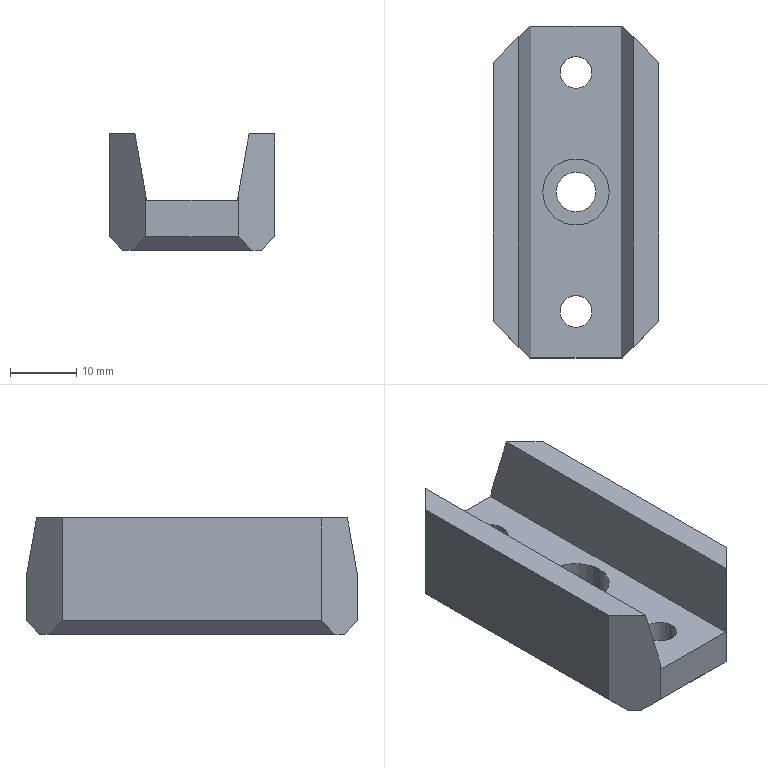Part | Creo | 1 solid | 27 faces | box 25 x 50 x 17.5 mm | volume 12117 mm3 | plane 19 | cylinder 8 | commonest cylinder face diameters 4.8 x4 6 x2 10 x2
STEP:
#1=CARTESIAN_POINT('',(-137.,25.,29.153));
#2=VERTEX_POINT('',#1);
#3=CARTESIAN_POINT('',(-136.825,25.,28.161));
#4=VERTEX_POINT('',#3);
#5=CARTESIAN_POINT('',(-137.,25.,29.153));
#6=DIRECTION('',(0.1736,0.,-0.9848));
#7=VECTOR('',#6,1.008);
#8=LINE('',#5,#7);
#9=EDGE_CURVE('',#2,#4,#8,.T.);
#10=ORIENTED_EDGE('',*,*,#9,.T.);
#11=CARTESIAN_POINT('',(-136.825,-25.,28.161));
#12=VERTEX_POINT('',#11);
#13=CARTESIAN_POINT('',(-136.825,-25.,28.161));
#14=DIRECTION('',(0.,1.,0.));
#15=VECTOR('',#14,50.);
#16=LINE('',#13,#15);
#17=EDGE_CURVE('',#12,#4,#16,.T.);
#18=ORIENTED_EDGE('',*,*,#17,.F.);
#19=CARTESIAN_POINT('',(-137.,-25.,29.153));
#20=VERTEX_POINT('',#19);
#21=CARTESIAN_POINT('',(-136.825,-25.,28.161));
#22=DIRECTION('',(-0.1736,0.,0.9848));
#23=VECTOR('',#22,1.008);
#24=LINE('',#21,#23);
#25=EDGE_CURVE('',#12,#20,#24,.T.);
#26=ORIENTED_EDGE('',*,*,#25,.T.);
#27=CARTESIAN_POINT('',(-138.588,-23.412,38.161));
#28=VERTEX_POINT('',#27);
#29=CARTESIAN_POINT('',(-138.588,-23.412,38.161));
#30=DIRECTION('',(0.1711,-0.1711,-0.9703));
#31=VECTOR('',#30,9.283);
#32=LINE('',#29,#31);
#33=EDGE_CURVE('',#28,#20,#32,.T.);
#34=ORIENTED_EDGE('',*,*,#33,.F.);
#35=CARTESIAN_POINT('',(-138.588,23.412,38.161));
#36=VERTEX_POINT('',#35);
#37=CARTESIAN_POINT('',(-138.588,-23.412,38.161));
#38=DIRECTION('',(0.,1.,0.));
#39=VECTOR('',#38,46.823);
#40=LINE('',#37,#39);
#41=EDGE_CURVE('',#28,#36,#40,.T.);
#42=ORIENTED_EDGE('',*,*,#41,.T.);
#43=CARTESIAN_POINT('',(-137.,25.,29.153));
#44=DIRECTION('',(-0.1711,-0.1711,0.9703));
#45=VECTOR('',#44,9.283);
#46=LINE('',#43,#45);
#47=EDGE_CURVE('',#2,#36,#46,.T.);
#48=ORIENTED_EDGE('',*,*,#47,.F.);
#49=EDGE_LOOP('',(#10,#18,#26,#34,#42,#48));
#50=FACE_OUTER_BOUND('',#49,.F.);
#51=CARTESIAN_POINT('',(-136.825,50.,28.161));
#52=DIRECTION('',(0.9848,0.,0.1736));
#53=DIRECTION('',(-0.1736,0.,0.9848));
#54=AXIS2_PLACEMENT_3D('',#51,#52,#53);
#55=PLANE('',#54);
#56=ADVANCED_FACE('',(#50),#55,.T.);
#57=CARTESIAN_POINT('',(-123.175,25.,28.161));
#58=VERTEX_POINT('',#57);
#59=CARTESIAN_POINT('',(-123.175,25.,28.161));
#60=DIRECTION('',(-1.,0.,0.));
#61=VECTOR('',#60,13.65);
#62=LINE('',#59,#61);
#63=EDGE_CURVE('',#58,#4,#62,.T.);
#64=ORIENTED_EDGE('',*,*,#63,.T.);
#65=ORIENTED_EDGE('',*,*,#9,.F.);
#66=CARTESIAN_POINT('',(-137.,25.,22.661));
#67=VERTEX_POINT('',#66);
#68=CARTESIAN_POINT('',(-137.,25.,29.153));
#69=DIRECTION('',(0.,0.,-1.));
#70=VECTOR('',#69,6.492);
#71=LINE('',#68,#70);
#72=EDGE_CURVE('',#2,#67,#71,.T.);
#73=ORIENTED_EDGE('',*,*,#72,.T.);
#74=CARTESIAN_POINT('',(-123.,25.,22.661));
#75=VERTEX_POINT('',#74);
#76=CARTESIAN_POINT('',(-137.,25.,22.661));
#77=DIRECTION('',(1.,0.,0.));
#78=VECTOR('',#77,14.);
#79=LINE('',#76,#78);
#80=EDGE_CURVE('',#67,#75,#79,.T.);
#81=ORIENTED_EDGE('',*,*,#80,.T.);
#82=CARTESIAN_POINT('',(-123.,25.,29.153));
#83=VERTEX_POINT('',#82);
#84=CARTESIAN_POINT('',(-123.,25.,22.661));
#85=DIRECTION('',(0.,0.,1.));
#86=VECTOR('',#85,6.492);
#87=LINE('',#84,#86);
#88=EDGE_CURVE('',#75,#83,#87,.T.);
#89=ORIENTED_EDGE('',*,*,#88,.T.);
#90=CARTESIAN_POINT('',(-123.175,25.,28.161));
#91=DIRECTION('',(0.1736,0.,0.9848));
#92=VECTOR('',#91,1.008);
#93=LINE('',#90,#92);
#94=EDGE_CURVE('',#58,#83,#93,.T.);
#95=ORIENTED_EDGE('',*,*,#94,.F.);
#96=EDGE_LOOP('',(#64,#65,#73,#81,#89,#95));
#97=FACE_OUTER_BOUND('',#96,.F.);
#98=CARTESIAN_POINT('',(-117.5,25.,46.161));
#99=DIRECTION('',(0.,1.,0.));
#100=DIRECTION('',(-1.,0.,0.));
#101=AXIS2_PLACEMENT_3D('',#98,#99,#100);
#102=PLANE('',#101);
#103=ADVANCED_FACE('',(#97),#102,.T.);
#104=ORIENTED_EDGE('',*,*,#17,.T.);
#105=ORIENTED_EDGE('',*,*,#63,.F.);
#106=CARTESIAN_POINT('',(-123.175,-25.,28.161));
#107=VERTEX_POINT('',#106);
#108=CARTESIAN_POINT('',(-123.175,-25.,28.161));
#109=DIRECTION('',(0.,1.,0.));
#110=VECTOR('',#109,50.);
#111=LINE('',#108,#110);
#112=EDGE_CURVE('',#107,#58,#111,.T.);
#113=ORIENTED_EDGE('',*,*,#112,.F.);
#114=CARTESIAN_POINT('',(-123.175,-25.,28.161));
#115=DIRECTION('',(-1.,0.,0.));
#116=VECTOR('',#115,13.65);
#117=LINE('',#114,#116);
#118=EDGE_CURVE('',#107,#12,#117,.T.);
#119=ORIENTED_EDGE('',*,*,#118,.T.);
#120=EDGE_LOOP('',(#104,#105,#113,#119));
#121=FACE_OUTER_BOUND('',#120,.F.);
#122=CARTESIAN_POINT('',(-132.4,18.,28.161));
#123=VERTEX_POINT('',#122);
#124=CARTESIAN_POINT('',(-127.6,18.,28.161));
#125=VERTEX_POINT('',#124);
#126=CARTESIAN_POINT('',(-130.,18.,28.161));
#127=DIRECTION('',(0.,0.,-1.));
#128=DIRECTION('',(-1.,0.,0.));
#129=AXIS2_PLACEMENT_3D('',#126,#127,#128);
#130=CIRCLE('',#129,2.4);
#131=EDGE_CURVE('',#123,#125,#130,.T.);
#132=ORIENTED_EDGE('',*,*,#131,.F.);
#133=CARTESIAN_POINT('',(-130.,18.,28.161));
#134=DIRECTION('',(0.,0.,-1.));
#135=DIRECTION('',(1.,0.,0.));
#136=AXIS2_PLACEMENT_3D('',#133,#134,#135);
#137=CIRCLE('',#136,2.4);
#138=EDGE_CURVE('',#125,#123,#137,.T.);
#139=ORIENTED_EDGE('',*,*,#138,.F.);
#140=EDGE_LOOP('',(#132,#139));
#141=FACE_BOUND('',#140,.F.);
#142=CARTESIAN_POINT('',(-132.4,-18.,28.161));
#143=VERTEX_POINT('',#142);
#144=CARTESIAN_POINT('',(-127.6,-18.,28.161));
#145=VERTEX_POINT('',#144);
#146=CARTESIAN_POINT('',(-130.,-18.,28.161));
#147=DIRECTION('',(0.,0.,-1.));
#148=DIRECTION('',(-1.,0.,0.));
#149=AXIS2_PLACEMENT_3D('',#146,#147,#148);
#150=CIRCLE('',#149,2.4);
#151=EDGE_CURVE('',#143,#145,#150,.T.);
#152=ORIENTED_EDGE('',*,*,#151,.F.);
#153=CARTESIAN_POINT('',(-130.,-18.,28.161));
#154=DIRECTION('',(0.,0.,-1.));
#155=DIRECTION('',(1.,0.,0.));
#156=AXIS2_PLACEMENT_3D('',#153,#154,#155);
#157=CIRCLE('',#156,2.4);
#158=EDGE_CURVE('',#145,#143,#157,.T.);
#159=ORIENTED_EDGE('',*,*,#158,.F.);
#160=EDGE_LOOP('',(#152,#159));
#161=FACE_BOUND('',#160,.F.);
#162=CARTESIAN_POINT('',(-125.,0.,28.161));
#163=VERTEX_POINT('',#162);
#164=CARTESIAN_POINT('',(-135.,0.,28.161));
#165=VERTEX_POINT('',#164);
#166=CARTESIAN_POINT('',(-130.,0.,28.161));
#167=DIRECTION('',(0.,0.,-1.));
#168=DIRECTION('',(1.,0.,0.));
#169=AXIS2_PLACEMENT_3D('',#166,#167,#168);
#170=CIRCLE('',#169,5.);
#171=EDGE_CURVE('',#163,#165,#170,.T.);
#172=ORIENTED_EDGE('',*,*,#171,.F.);
#173=CARTESIAN_POINT('',(-130.,0.,28.161));
#174=DIRECTION('',(0.,0.,-1.));
#175=DIRECTION('',(-1.,0.,0.));
#176=AXIS2_PLACEMENT_3D('',#173,#174,#175);
#177=CIRCLE('',#176,5.);
#178=EDGE_CURVE('',#165,#163,#177,.T.);
#179=ORIENTED_EDGE('',*,*,#178,.F.);
#180=EDGE_LOOP('',(#172,#179));
#181=FACE_BOUND('',#180,.F.);
#182=CARTESIAN_POINT('',(-123.175,50.,28.161));
#183=DIRECTION('',(0.,0.,1.));
#184=DIRECTION('',(-1.,0.,0.));
#185=AXIS2_PLACEMENT_3D('',#182,#183,#184);
#186=PLANE('',#185);
#187=ADVANCED_FACE('',(#121,#141,#161,#181),#186,.T.);
#188=CARTESIAN_POINT('',(-135.,0.,22.161));
#189=VERTEX_POINT('',#188);
#190=CARTESIAN_POINT('',(-125.,0.,22.161));
#191=VERTEX_POINT('',#190);
#192=CARTESIAN_POINT('',(-130.,0.,22.161));
#193=DIRECTION('',(0.,0.,1.));
#194=DIRECTION('',(-1.,0.,0.));
#195=AXIS2_PLACEMENT_3D('',#192,#193,#194);
#196=CIRCLE('',#195,5.);
#197=EDGE_CURVE('',#189,#191,#196,.T.);
#198=ORIENTED_EDGE('',*,*,#197,.T.);
#199=CARTESIAN_POINT('',(-125.,0.,28.161));
#200=DIRECTION('',(0.,0.,-1.));
#201=VECTOR('',#200,6.);
#202=LINE('',#199,#201);
#203=EDGE_CURVE('',#163,#191,#202,.T.);
#204=ORIENTED_EDGE('',*,*,#203,.F.);
#205=ORIENTED_EDGE('',*,*,#171,.T.);
#206=CARTESIAN_POINT('',(-135.,0.,28.161));
#207=DIRECTION('',(0.,0.,-1.));
#208=VECTOR('',#207,6.);
#209=LINE('',#206,#208);
#210=EDGE_CURVE('',#165,#189,#209,.T.);
#211=ORIENTED_EDGE('',*,*,#210,.T.);
#212=EDGE_LOOP('',(#198,#204,#205,#211));
#213=FACE_OUTER_BOUND('',#212,.F.);
#214=CARTESIAN_POINT('',(-130.,0.,28.161));
#215=DIRECTION('',(0.,0.,-1.));
#216=DIRECTION('',(1.,0.,0.));
#217=AXIS2_PLACEMENT_3D('',#214,#215,#216);
#218=CYLINDRICAL_SURFACE('',#217,5.);
#219=ADVANCED_FACE('',(#213),#218,.F.);
#220=CARTESIAN_POINT('',(-130.,0.,22.161));
#221=DIRECTION('',(0.,0.,1.));
#222=DIRECTION('',(1.,0.,0.));
#223=AXIS2_PLACEMENT_3D('',#220,#221,#222);
#224=CIRCLE('',#223,5.);
#225=EDGE_CURVE('',#191,#189,#224,.T.);
#226=ORIENTED_EDGE('',*,*,#225,.F.);
#227=ORIENTED_EDGE('',*,*,#197,.F.);
#228=EDGE_LOOP('',(#226,#227));
#229=FACE_OUTER_BOUND('',#228,.F.);
#230=CARTESIAN_POINT('',(-127.,0.,22.161));
#231=VERTEX_POINT('',#230);
#232=CARTESIAN_POINT('',(-133.,0.,22.161));
#233=VERTEX_POINT('',#232);
#234=CARTESIAN_POINT('',(-130.,0.,22.161));
#235=DIRECTION('',(0.,0.,-1.));
#236=DIRECTION('',(1.,0.,0.));
#237=AXIS2_PLACEMENT_3D('',#234,#235,#236);
#238=CIRCLE('',#237,3.);
#239=EDGE_CURVE('',#231,#233,#238,.T.);
#240=ORIENTED_EDGE('',*,*,#239,.F.);
#241=CARTESIAN_POINT('',(-130.,0.,22.161));
#242=DIRECTION('',(0.,0.,-1.));
#243=DIRECTION('',(-1.,0.,0.));
#244=AXIS2_PLACEMENT_3D('',#241,#242,#243);
#245=CIRCLE('',#244,3.);
#246=EDGE_CURVE('',#233,#231,#245,.T.);
#247=ORIENTED_EDGE('',*,*,#246,.F.);
#248=EDGE_LOOP('',(#240,#247));
#249=FACE_BOUND('',#248,.F.);
#250=CARTESIAN_POINT('',(-130.,0.,22.161));
#251=DIRECTION('',(0.,0.,-1.));
#252=DIRECTION('',(1.,0.,0.));
#253=AXIS2_PLACEMENT_3D('',#250,#251,#252);
#254=PLANE('',#253);
#255=ADVANCED_FACE('',(#229,#249),#254,.F.);
#256=ORIENTED_EDGE('',*,*,#225,.T.);
#257=ORIENTED_EDGE('',*,*,#210,.F.);
#258=ORIENTED_EDGE('',*,*,#178,.T.);
#259=ORIENTED_EDGE('',*,*,#203,.T.);
#260=EDGE_LOOP('',(#256,#257,#258,#259));
#261=FACE_OUTER_BOUND('',#260,.F.);
#262=CARTESIAN_POINT('',(-130.,0.,28.161));
#263=DIRECTION('',(0.,0.,-1.));
#264=DIRECTION('',(1.,0.,0.));
#265=AXIS2_PLACEMENT_3D('',#262,#263,#264);
#266=CYLINDRICAL_SURFACE('',#265,5.);
#267=ADVANCED_FACE('',(#261),#266,.F.);
#268=ORIENTED_EDGE('',*,*,#239,.T.);
#269=CARTESIAN_POINT('',(-133.,0.,20.661));
#270=VERTEX_POINT('',#269);
#271=CARTESIAN_POINT('',(-133.,0.,22.161));
#272=DIRECTION('',(0.,0.,-1.));
#273=VECTOR('',#272,1.5);
#274=LINE('',#271,#273);
#275=EDGE_CURVE('',#233,#270,#274,.T.);
#276=ORIENTED_EDGE('',*,*,#275,.T.);
#277=CARTESIAN_POINT('',(-127.,0.,20.661));
#278=VERTEX_POINT('',#277);
#279=CARTESIAN_POINT('',(-130.,0.,20.661));
#280=DIRECTION('',(0.,0.,1.));
#281=DIRECTION('',(-1.,0.,0.));
#282=AXIS2_PLACEMENT_3D('',#279,#280,#281);
#283=CIRCLE('',#282,3.);
#284=EDGE_CURVE('',#270,#278,#283,.T.);
#285=ORIENTED_EDGE('',*,*,#284,.T.);
#286=CARTESIAN_POINT('',(-127.,0.,22.161));
#287=DIRECTION('',(0.,0.,-1.));
#288=VECTOR('',#287,1.5);
#289=LINE('',#286,#288);
#290=EDGE_CURVE('',#231,#278,#289,.T.);
#291=ORIENTED_EDGE('',*,*,#290,.F.);
#292=EDGE_LOOP('',(#268,#276,#285,#291));
#293=FACE_OUTER_BOUND('',#292,.F.);
#294=CARTESIAN_POINT('',(-130.,0.,46.161));
#295=DIRECTION('',(0.,0.,-1.));
#296=DIRECTION('',(1.,0.,0.));
#297=AXIS2_PLACEMENT_3D('',#294,#295,#296);
#298=CYLINDRICAL_SURFACE('',#297,3.);
#299=ADVANCED_FACE('',(#293),#298,.F.);
#300=ORIENTED_EDGE('',*,*,#246,.T.);
#301=ORIENTED_EDGE('',*,*,#290,.T.);
#302=CARTESIAN_POINT('',(-130.,0.,20.661));
#303=DIRECTION('',(0.,0.,1.));
#304=DIRECTION('',(1.,0.,0.));
#305=AXIS2_PLACEMENT_3D('',#302,#303,#304);
#306=CIRCLE('',#305,3.);
#307=EDGE_CURVE('',#278,#270,#306,.T.);
#308=ORIENTED_EDGE('',*,*,#307,.T.);
#309=ORIENTED_EDGE('',*,*,#275,.F.);
#310=EDGE_LOOP('',(#300,#301,#308,#309));
#311=FACE_OUTER_BOUND('',#310,.F.);
#312=CARTESIAN_POINT('',(-130.,0.,46.161));
#313=DIRECTION('',(0.,0.,-1.));
#314=DIRECTION('',(1.,0.,0.));
#315=AXIS2_PLACEMENT_3D('',#312,#313,#314);
#316=CYLINDRICAL_SURFACE('',#315,3.);
#317=ADVANCED_FACE('',(#311),#316,.F.);
#318=CARTESIAN_POINT('',(-121.,23.,20.661));
#319=VERTEX_POINT('',#318);
#320=CARTESIAN_POINT('',(-139.,23.,20.661));
#321=VERTEX_POINT('',#320);
#322=CARTESIAN_POINT('',(-121.,23.,20.661));
#323=DIRECTION('',(-1.,0.,0.));
#324=VECTOR('',#323,18.);
#325=LINE('',#322,#324);
#326=EDGE_CURVE('',#319,#321,#325,.T.);
#327=ORIENTED_EDGE('',*,*,#326,.T.);
#328=CARTESIAN_POINT('',(-140.5,21.5,20.661));
#329=VERTEX_POINT('',#328);
#330=CARTESIAN_POINT('',(-140.5,21.5,20.661));
#331=DIRECTION('',(0.7071,0.7071,0.));
#332=VECTOR('',#331,2.121);
#333=LINE('',#330,#332);
#334=EDGE_CURVE('',#329,#321,#333,.T.);
#335=ORIENTED_EDGE('',*,*,#334,.F.);
#336=CARTESIAN_POINT('',(-140.5,-21.5,20.661));
#337=VERTEX_POINT('',#336);
#338=CARTESIAN_POINT('',(-140.5,21.5,20.661));
#339=DIRECTION('',(0.,-1.,0.));
#340=VECTOR('',#339,43.);
#341=LINE('',#338,#340);
#342=EDGE_CURVE('',#329,#337,#341,.T.);
#343=ORIENTED_EDGE('',*,*,#342,.T.);
#344=CARTESIAN_POINT('',(-139.,-23.,20.661));
#345=VERTEX_POINT('',#344);
#346=CARTESIAN_POINT('',(-139.,-23.,20.661));
#347=DIRECTION('',(-0.7071,0.7071,0.));
#348=VECTOR('',#347,2.121);
#349=LINE('',#346,#348);
#350=EDGE_CURVE('',#345,#337,#349,.T.);
#351=ORIENTED_EDGE('',*,*,#350,.F.);
#352=CARTESIAN_POINT('',(-121.,-23.,20.661));
#353=VERTEX_POINT('',#352);
#354=CARTESIAN_POINT('',(-139.,-23.,20.661));
#355=DIRECTION('',(1.,0.,0.));
#356=VECTOR('',#355,18.);
#357=LINE('',#354,#356);
#358=EDGE_CURVE('',#345,#353,#357,.T.);
#359=ORIENTED_EDGE('',*,*,#358,.T.);
#360=CARTESIAN_POINT('',(-119.5,-21.5,20.661));
#361=VERTEX_POINT('',#360);
#362=CARTESIAN_POINT('',(-119.5,-21.5,20.661));
#363=DIRECTION('',(-0.7071,-0.7071,0.));
#364=VECTOR('',#363,2.121);
#365=LINE('',#362,#364);
#366=EDGE_CURVE('',#361,#353,#365,.T.);
#367=ORIENTED_EDGE('',*,*,#366,.F.);
#368=CARTESIAN_POINT('',(-119.5,21.5,20.661));
#369=VERTEX_POINT('',#368);
#370=CARTESIAN_POINT('',(-119.5,-21.5,20.661));
#371=DIRECTION('',(0.,1.,0.));
#372=VECTOR('',#371,43.);
#373=LINE('',#370,#372);
#374=EDGE_CURVE('',#361,#369,#373,.T.);
#375=ORIENTED_EDGE('',*,*,#374,.T.);
#376=CARTESIAN_POINT('',(-121.,23.,20.661));
#377=DIRECTION('',(0.7071,-0.7071,0.));
#378=VECTOR('',#377,2.121);
#379=LINE('',#376,#378);
#380=EDGE_CURVE('',#319,#369,#379,.T.);
#381=ORIENTED_EDGE('',*,*,#380,.F.);
#382=EDGE_LOOP('',(#327,#335,#343,#351,#359,#367,#375,#381));
#383=FACE_OUTER_BOUND('',#382,.F.);
#384=CARTESIAN_POINT('',(-132.4,-18.,20.661));
#385=VERTEX_POINT('',#384);
#386=CARTESIAN_POINT('',(-127.6,-18.,20.661));
#387=VERTEX_POINT('',#386);
#388=CARTESIAN_POINT('',(-130.,-18.,20.661));
#389=DIRECTION('',(0.,0.,1.));
#390=DIRECTION('',(-1.,0.,0.));
#391=AXIS2_PLACEMENT_3D('',#388,#389,#390);
#392=CIRCLE('',#391,2.4);
#393=EDGE_CURVE('',#385,#387,#392,.T.);
#394=ORIENTED_EDGE('',*,*,#393,.F.);
#395=CARTESIAN_POINT('',(-130.,-18.,20.661));
#396=DIRECTION('',(0.,0.,1.));
#397=DIRECTION('',(1.,0.,0.));
#398=AXIS2_PLACEMENT_3D('',#395,#396,#397);
#399=CIRCLE('',#398,2.4);
#400=EDGE_CURVE('',#387,#385,#399,.T.);
#401=ORIENTED_EDGE('',*,*,#400,.F.);
#402=EDGE_LOOP('',(#394,#401));
#403=FACE_BOUND('',#402,.F.);
#404=ORIENTED_EDGE('',*,*,#284,.F.);
#405=ORIENTED_EDGE('',*,*,#307,.F.);
#406=EDGE_LOOP('',(#404,#405));
#407=FACE_BOUND('',#406,.F.);
#408=CARTESIAN_POINT('',(-132.4,18.,20.661));
#409=VERTEX_POINT('',#408);
#410=CARTESIAN_POINT('',(-127.6,18.,20.661));
#411=VERTEX_POINT('',#410);
#412=CARTESIAN_POINT('',(-130.,18.,20.661));
#413=DIRECTION('',(0.,0.,1.));
#414=DIRECTION('',(-1.,0.,0.));
#415=AXIS2_PLACEMENT_3D('',#412,#413,#414);
#416=CIRCLE('',#415,2.4);
#417=EDGE_CURVE('',#409,#411,#416,.T.);
#418=ORIENTED_EDGE('',*,*,#417,.F.);
#419=CARTESIAN_POINT('',(-130.,18.,20.661));
#420=DIRECTION('',(0.,0.,1.));
#421=DIRECTION('',(1.,0.,0.));
#422=AXIS2_PLACEMENT_3D('',#419,#420,#421);
#423=CIRCLE('',#422,2.4);
#424=EDGE_CURVE('',#411,#409,#423,.T.);
#425=ORIENTED_EDGE('',*,*,#424,.F.);
#426=EDGE_LOOP('',(#418,#425));
#427=FACE_BOUND('',#426,.F.);
#428=CARTESIAN_POINT('',(-142.5,-25.,20.661));
#429=DIRECTION('',(0.,0.,1.));
#430=DIRECTION('',(-1.,0.,0.));
#431=AXIS2_PLACEMENT_3D('',#428,#429,#430);
#432=PLANE('',#431);
#433=ADVANCED_FACE('',(#383,#403,#407,#427),#432,.F.);
#434=ORIENTED_EDGE('',*,*,#417,.T.);
#435=CARTESIAN_POINT('',(-127.6,18.,28.161));
#436=DIRECTION('',(0.,0.,-1.));
#437=VECTOR('',#436,7.5);
#438=LINE('',#435,#437);
#439=EDGE_CURVE('',#125,#411,#438,.T.);
#440=ORIENTED_EDGE('',*,*,#439,.F.);
#441=ORIENTED_EDGE('',*,*,#138,.T.);
#442=CARTESIAN_POINT('',(-132.4,18.,28.161));
#443=DIRECTION('',(0.,0.,-1.));
#444=VECTOR('',#443,7.5);
#445=LINE('',#442,#444);
#446=EDGE_CURVE('',#123,#409,#445,.T.);
#447=ORIENTED_EDGE('',*,*,#446,.T.);
#448=EDGE_LOOP('',(#434,#440,#441,#447));
#449=FACE_OUTER_BOUND('',#448,.F.);
#450=CARTESIAN_POINT('',(-130.,18.,46.161));
#451=DIRECTION('',(0.,0.,-1.));
#452=DIRECTION('',(1.,0.,0.));
#453=AXIS2_PLACEMENT_3D('',#450,#451,#452);
#454=CYLINDRICAL_SURFACE('',#453,2.4);
#455=ADVANCED_FACE('',(#449),#454,.F.);
#456=ORIENTED_EDGE('',*,*,#424,.T.);
#457=ORIENTED_EDGE('',*,*,#446,.F.);
#458=ORIENTED_EDGE('',*,*,#131,.T.);
#459=ORIENTED_EDGE('',*,*,#439,.T.);
#460=EDGE_LOOP('',(#456,#457,#458,#459));
#461=FACE_OUTER_BOUND('',#460,.F.);
#462=CARTESIAN_POINT('',(-130.,18.,46.161));
#463=DIRECTION('',(0.,0.,-1.));
#464=DIRECTION('',(1.,0.,0.));
#465=AXIS2_PLACEMENT_3D('',#462,#463,#464);
#466=CYLINDRICAL_SURFACE('',#465,2.4);
#467=ADVANCED_FACE('',(#461),#466,.F.);
#468=ORIENTED_EDGE('',*,*,#393,.T.);
#469=CARTESIAN_POINT('',(-127.6,-18.,28.161));
#470=DIRECTION('',(0.,0.,-1.));
#471=VECTOR('',#470,7.5);
#472=LINE('',#469,#471);
#473=EDGE_CURVE('',#145,#387,#472,.T.);
#474=ORIENTED_EDGE('',*,*,#473,.F.);
#475=ORIENTED_EDGE('',*,*,#158,.T.);
#476=CARTESIAN_POINT('',(-132.4,-18.,28.161));
#477=DIRECTION('',(0.,0.,-1.));
#478=VECTOR('',#477,7.5);
#479=LINE('',#476,#478);
#480=EDGE_CURVE('',#143,#385,#479,.T.);
#481=ORIENTED_EDGE('',*,*,#480,.T.);
#482=EDGE_LOOP('',(#468,#474,#475,#481));
#483=FACE_OUTER_BOUND('',#482,.F.);
#484=CARTESIAN_POINT('',(-130.,-18.,46.161));
#485=DIRECTION('',(0.,0.,-1.));
#486=DIRECTION('',(1.,0.,0.));
#487=AXIS2_PLACEMENT_3D('',#484,#485,#486);
#488=CYLINDRICAL_SURFACE('',#487,2.4);
#489=ADVANCED_FACE('',(#483),#488,.F.);
#490=ORIENTED_EDGE('',*,*,#400,.T.);
#491=ORIENTED_EDGE('',*,*,#480,.F.);
#492=ORIENTED_EDGE('',*,*,#151,.T.);
#493=ORIENTED_EDGE('',*,*,#473,.T.);
#494=EDGE_LOOP('',(#490,#491,#492,#493));
#495=FACE_OUTER_BOUND('',#494,.F.);
#496=CARTESIAN_POINT('',(-130.,-18.,46.161));
#497=DIRECTION('',(0.,0.,-1.));
#498=DIRECTION('',(1.,0.,0.));
#499=AXIS2_PLACEMENT_3D('',#496,#497,#498);
#500=CYLINDRICAL_SURFACE('',#499,2.4);
#501=ADVANCED_FACE('',(#495),#500,.F.);
#502=ORIENTED_EDGE('',*,*,#80,.F.);
#503=CARTESIAN_POINT('',(-137.,25.,22.661));
#504=DIRECTION('',(-0.5774,-0.5774,-0.5774));
#505=VECTOR('',#504,3.464);
#506=LINE('',#503,#505);
#507=EDGE_CURVE('',#67,#321,#506,.T.);
#508=ORIENTED_EDGE('',*,*,#507,.T.);
#509=ORIENTED_EDGE('',*,*,#326,.F.);
#510=CARTESIAN_POINT('',(-121.,23.,20.661));
#511=DIRECTION('',(-0.5774,0.5774,0.5774));
#512=VECTOR('',#511,3.464);
#513=LINE('',#510,#512);
#514=EDGE_CURVE('',#319,#75,#513,.T.);
#515=ORIENTED_EDGE('',*,*,#514,.T.);
#516=EDGE_LOOP('',(#502,#508,#509,#515));
#517=FACE_OUTER_BOUND('',#516,.F.);
#518=CARTESIAN_POINT('',(-142.5,23.,20.661));
#519=DIRECTION('',(0.,0.7071,-0.7071));
#520=DIRECTION('',(0.,-0.7071,-0.7071));
#521=AXIS2_PLACEMENT_3D('',#518,#519,#520);
#522=PLANE('',#521);
#523=ADVANCED_FACE('',(#517),#522,.T.);
#524=CARTESIAN_POINT('',(-142.5,19.5,38.161));
#525=VERTEX_POINT('',#524);
#526=CARTESIAN_POINT('',(-138.588,23.412,38.161));
#527=DIRECTION('',(-0.7071,-0.7071,0.));
#528=VECTOR('',#527,5.532);
#529=LINE('',#526,#528);
#530=EDGE_CURVE('',#36,#525,#529,.T.);
#531=ORIENTED_EDGE('',*,*,#530,.T.);
#532=CARTESIAN_POINT('',(-142.5,19.5,22.661));
#533=VERTEX_POINT('',#532);
#534=CARTESIAN_POINT('',(-142.5,19.5,22.661));
#535=DIRECTION('',(0.,0.,1.));
#536=VECTOR('',#535,15.5);
#537=LINE('',#534,#536);
#538=EDGE_CURVE('',#533,#525,#537,.T.);
#539=ORIENTED_EDGE('',*,*,#538,.F.);
#540=CARTESIAN_POINT('',(-140.5,21.5,20.661));
#541=DIRECTION('',(-0.5774,-0.5774,0.5774));
#542=VECTOR('',#541,3.464);
#543=LINE('',#540,#542);
#544=EDGE_CURVE('',#329,#533,#543,.T.);
#545=ORIENTED_EDGE('',*,*,#544,.F.);
#546=ORIENTED_EDGE('',*,*,#334,.T.);
#547=ORIENTED_EDGE('',*,*,#507,.F.);
#548=ORIENTED_EDGE('',*,*,#72,.F.);
#549=ORIENTED_EDGE('',*,*,#47,.T.);
#550=EDGE_LOOP('',(#531,#539,#545,#546,#547,#548,#549));
#551=FACE_OUTER_BOUND('',#550,.F.);
#552=CARTESIAN_POINT('',(-142.5,19.5,38.161));
#553=DIRECTION('',(-0.7071,0.7071,0.));
#554=DIRECTION('',(-0.7071,-0.7071,0.));
#555=AXIS2_PLACEMENT_3D('',#552,#553,#554);
#556=PLANE('',#555);
#557=ADVANCED_FACE('',(#551),#556,.T.);
#558=ORIENTED_EDGE('',*,*,#530,.F.);
#559=ORIENTED_EDGE('',*,*,#41,.F.);
#560=CARTESIAN_POINT('',(-142.5,-19.5,38.161));
#561=VERTEX_POINT('',#560);
#562=CARTESIAN_POINT('',(-142.5,-19.5,38.161));
#563=DIRECTION('',(0.7071,-0.7071,0.));
#564=VECTOR('',#563,5.532);
#565=LINE('',#562,#564);
#566=EDGE_CURVE('',#561,#28,#565,.T.);
#567=ORIENTED_EDGE('',*,*,#566,.F.);
#568=CARTESIAN_POINT('',(-142.5,-19.5,38.161));
#569=DIRECTION('',(0.,1.,0.));
#570=VECTOR('',#569,39.);
#571=LINE('',#568,#570);
#572=EDGE_CURVE('',#561,#525,#571,.T.);
#573=ORIENTED_EDGE('',*,*,#572,.T.);
#574=EDGE_LOOP('',(#558,#559,#567,#573));
#575=FACE_OUTER_BOUND('',#574,.F.);
#576=CARTESIAN_POINT('',(-138.588,50.,38.161));
#577=DIRECTION('',(0.,0.,1.));
#578=DIRECTION('',(-1.,0.,0.));
#579=AXIS2_PLACEMENT_3D('',#576,#577,#578);
#580=PLANE('',#579);
#581=ADVANCED_FACE('',(#575),#580,.T.);
#582=CARTESIAN_POINT('',(-137.,-25.,22.661));
#583=VERTEX_POINT('',#582);
#584=CARTESIAN_POINT('',(-137.,-25.,22.661));
#585=DIRECTION('',(0.,0.,1.));
#586=VECTOR('',#585,6.492);
#587=LINE('',#584,#586);
#588=EDGE_CURVE('',#583,#20,#587,.T.);
#589=ORIENTED_EDGE('',*,*,#588,.F.);
#590=CARTESIAN_POINT('',(-139.,-23.,20.661));
#591=DIRECTION('',(0.5774,-0.5774,0.5774));
#592=VECTOR('',#591,3.464);
#593=LINE('',#590,#592);
#594=EDGE_CURVE('',#345,#583,#593,.T.);
#595=ORIENTED_EDGE('',*,*,#594,.F.);
#596=ORIENTED_EDGE('',*,*,#350,.T.);
#597=CARTESIAN_POINT('',(-142.5,-19.5,22.661));
#598=VERTEX_POINT('',#597);
#599=CARTESIAN_POINT('',(-142.5,-19.5,22.661));
#600=DIRECTION('',(0.5774,-0.5774,-0.5774));
#601=VECTOR('',#600,3.464);
#602=LINE('',#599,#601);
#603=EDGE_CURVE('',#598,#337,#602,.T.);
#604=ORIENTED_EDGE('',*,*,#603,.F.);
#605=CARTESIAN_POINT('',(-142.5,-19.5,38.161));
#606=DIRECTION('',(0.,0.,-1.));
#607=VECTOR('',#606,15.5);
#608=LINE('',#605,#607);
#609=EDGE_CURVE('',#561,#598,#608,.T.);
#610=ORIENTED_EDGE('',*,*,#609,.F.);
#611=ORIENTED_EDGE('',*,*,#566,.T.);
#612=ORIENTED_EDGE('',*,*,#33,.T.);
#613=EDGE_LOOP('',(#589,#595,#596,#604,#610,#611,#612));
#614=FACE_OUTER_BOUND('',#613,.F.);
#615=CARTESIAN_POINT('',(-137.,-25.,46.161));
#616=DIRECTION('',(0.7071,0.7071,0.));
#617=DIRECTION('',(-0.7071,0.7071,0.));
#618=AXIS2_PLACEMENT_3D('',#615,#616,#617);
#619=PLANE('',#618);
#620=ADVANCED_FACE('',(#614),#619,.F.);
#621=CARTESIAN_POINT('',(-123.,-25.,29.153));
#622=VERTEX_POINT('',#621);
#623=CARTESIAN_POINT('',(-123.,-25.,29.153));
#624=DIRECTION('',(-0.1736,0.,-0.9848));
#625=VECTOR('',#624,1.008);
#626=LINE('',#623,#625);
#627=EDGE_CURVE('',#622,#107,#626,.T.);
#628=ORIENTED_EDGE('',*,*,#627,.F.);
#629=CARTESIAN_POINT('',(-123.,-25.,22.661));
#630=VERTEX_POINT('',#629);
#631=CARTESIAN_POINT('',(-123.,-25.,29.153));
#632=DIRECTION('',(0.,0.,-1.));
#633=VECTOR('',#632,6.492);
#634=LINE('',#631,#633);
#635=EDGE_CURVE('',#622,#630,#634,.T.);
#636=ORIENTED_EDGE('',*,*,#635,.T.);
#637=CARTESIAN_POINT('',(-123.,-25.,22.661));
#638=DIRECTION('',(-1.,0.,0.));
#639=VECTOR('',#638,14.);
#640=LINE('',#637,#639);
#641=EDGE_CURVE('',#630,#583,#640,.T.);
#642=ORIENTED_EDGE('',*,*,#641,.T.);
#643=ORIENTED_EDGE('',*,*,#588,.T.);
#644=ORIENTED_EDGE('',*,*,#25,.F.);
#645=ORIENTED_EDGE('',*,*,#118,.F.);
#646=EDGE_LOOP('',(#628,#636,#642,#643,#644,#645));
#647=FACE_OUTER_BOUND('',#646,.F.);
#648=CARTESIAN_POINT('',(-117.5,-25.,46.161));
#649=DIRECTION('',(0.,1.,0.));
#650=DIRECTION('',(-1.,0.,0.));
#651=AXIS2_PLACEMENT_3D('',#648,#649,#650);
#652=PLANE('',#651);
#653=ADVANCED_FACE('',(#647),#652,.F.);
#654=ORIENTED_EDGE('',*,*,#94,.T.);
#655=CARTESIAN_POINT('',(-121.412,23.412,38.161));
#656=VERTEX_POINT('',#655);
#657=CARTESIAN_POINT('',(-121.412,23.412,38.161));
#658=DIRECTION('',(-0.1711,0.1711,-0.9703));
#659=VECTOR('',#658,9.283);
#660=LINE('',#657,#659);
#661=EDGE_CURVE('',#656,#83,#660,.T.);
#662=ORIENTED_EDGE('',*,*,#661,.F.);
#663=CARTESIAN_POINT('',(-121.412,-23.412,38.161));
#664=VERTEX_POINT('',#663);
#665=CARTESIAN_POINT('',(-121.412,-23.412,38.161));
#666=DIRECTION('',(0.,1.,0.));
#667=VECTOR('',#666,46.823);
#668=LINE('',#665,#667);
#669=EDGE_CURVE('',#664,#656,#668,.T.);
#670=ORIENTED_EDGE('',*,*,#669,.F.);
#671=CARTESIAN_POINT('',(-123.,-25.,29.153));
#672=DIRECTION('',(0.1711,0.1711,0.9703));
#673=VECTOR('',#672,9.283);
#674=LINE('',#671,#673);
#675=EDGE_CURVE('',#622,#664,#674,.T.);
#676=ORIENTED_EDGE('',*,*,#675,.F.);
#677=ORIENTED_EDGE('',*,*,#627,.T.);
#678=ORIENTED_EDGE('',*,*,#112,.T.);
#679=EDGE_LOOP('',(#654,#662,#670,#676,#677,#678));
#680=FACE_OUTER_BOUND('',#679,.F.);
#681=CARTESIAN_POINT('',(-121.412,50.,38.161));
#682=DIRECTION('',(-0.9848,0.,0.1736));
#683=DIRECTION('',(-0.1736,0.,-0.9848));
#684=AXIS2_PLACEMENT_3D('',#681,#682,#683);
#685=PLANE('',#684);
#686=ADVANCED_FACE('',(#680),#685,.T.);
#687=CARTESIAN_POINT('',(-117.5,19.5,38.161));
#688=VERTEX_POINT('',#687);
#689=CARTESIAN_POINT('',(-117.5,19.5,38.161));
#690=DIRECTION('',(-0.7071,0.7071,0.));
#691=VECTOR('',#690,5.532);
#692=LINE('',#689,#691);
#693=EDGE_CURVE('',#688,#656,#692,.T.);
#694=ORIENTED_EDGE('',*,*,#693,.T.);
#695=ORIENTED_EDGE('',*,*,#661,.T.);
#696=ORIENTED_EDGE('',*,*,#88,.F.);
#697=ORIENTED_EDGE('',*,*,#514,.F.);
#698=ORIENTED_EDGE('',*,*,#380,.T.);
#699=CARTESIAN_POINT('',(-117.5,19.5,22.661));
#700=VERTEX_POINT('',#699);
#701=CARTESIAN_POINT('',(-117.5,19.5,22.661));
#702=DIRECTION('',(-0.5774,0.5774,-0.5774));
#703=VECTOR('',#702,3.464);
#704=LINE('',#701,#703);
#705=EDGE_CURVE('',#700,#369,#704,.T.);
#706=ORIENTED_EDGE('',*,*,#705,.F.);
#707=CARTESIAN_POINT('',(-117.5,19.5,38.161));
#708=DIRECTION('',(0.,0.,-1.));
#709=VECTOR('',#708,15.5);
#710=LINE('',#707,#709);
#711=EDGE_CURVE('',#688,#700,#710,.T.);
#712=ORIENTED_EDGE('',*,*,#711,.F.);
#713=EDGE_LOOP('',(#694,#695,#696,#697,#698,#706,#712));
#714=FACE_OUTER_BOUND('',#713,.F.);
#715=CARTESIAN_POINT('',(-117.5,19.5,38.161));
#716=DIRECTION('',(0.7071,0.7071,0.));
#717=DIRECTION('',(-0.7071,0.7071,0.));
#718=AXIS2_PLACEMENT_3D('',#715,#716,#717);
#719=PLANE('',#718);
#720=ADVANCED_FACE('',(#714),#719,.T.);
#721=CARTESIAN_POINT('',(-117.5,-19.5,38.161));
#722=VERTEX_POINT('',#721);
#723=CARTESIAN_POINT('',(-117.5,-19.5,38.161));
#724=DIRECTION('',(0.,1.,0.));
#725=VECTOR('',#724,39.);
#726=LINE('',#723,#725);
#727=EDGE_CURVE('',#722,#688,#726,.T.);
#728=ORIENTED_EDGE('',*,*,#727,.F.);
#729=CARTESIAN_POINT('',(-121.412,-23.412,38.161));
#730=DIRECTION('',(0.7071,0.7071,0.));
#731=VECTOR('',#730,5.532);
#732=LINE('',#729,#731);
#733=EDGE_CURVE('',#664,#722,#732,.T.);
#734=ORIENTED_EDGE('',*,*,#733,.F.);
#735=ORIENTED_EDGE('',*,*,#669,.T.);
#736=ORIENTED_EDGE('',*,*,#693,.F.);
#737=EDGE_LOOP('',(#728,#734,#735,#736));
#738=FACE_OUTER_BOUND('',#737,.F.);
#739=CARTESIAN_POINT('',(-121.412,50.,38.161));
#740=DIRECTION('',(0.,0.,-1.));
#741=DIRECTION('',(1.,0.,0.));
#742=AXIS2_PLACEMENT_3D('',#739,#740,#741);
#743=PLANE('',#742);
#744=ADVANCED_FACE('',(#738),#743,.F.);
#745=ORIENTED_EDGE('',*,*,#711,.T.);
#746=CARTESIAN_POINT('',(-117.5,-19.5,22.661));
#747=VERTEX_POINT('',#746);
#748=CARTESIAN_POINT('',(-117.5,19.5,22.661));
#749=DIRECTION('',(0.,-1.,0.));
#750=VECTOR('',#749,39.);
#751=LINE('',#748,#750);
#752=EDGE_CURVE('',#700,#747,#751,.T.);
#753=ORIENTED_EDGE('',*,*,#752,.T.);
#754=CARTESIAN_POINT('',(-117.5,-19.5,22.661));
#755=DIRECTION('',(0.,0.,1.));
#756=VECTOR('',#755,15.5);
#757=LINE('',#754,#756);
#758=EDGE_CURVE('',#747,#722,#757,.T.);
#759=ORIENTED_EDGE('',*,*,#758,.T.);
#760=ORIENTED_EDGE('',*,*,#727,.T.);
#761=EDGE_LOOP('',(#745,#753,#759,#760));
#762=FACE_OUTER_BOUND('',#761,.F.);
#763=CARTESIAN_POINT('',(-117.5,-25.,38.161));
#764=DIRECTION('',(-1.,0.,0.));
#765=DIRECTION('',(0.,0.,-1.));
#766=AXIS2_PLACEMENT_3D('',#763,#764,#765);
#767=PLANE('',#766);
#768=ADVANCED_FACE('',(#762),#767,.F.);
#769=ORIENTED_EDGE('',*,*,#374,.F.);
#770=CARTESIAN_POINT('',(-119.5,-21.5,20.661));
#771=DIRECTION('',(0.5774,0.5774,0.5774));
#772=VECTOR('',#771,3.464);
#773=LINE('',#770,#772);
#774=EDGE_CURVE('',#361,#747,#773,.T.);
#775=ORIENTED_EDGE('',*,*,#774,.T.);
#776=ORIENTED_EDGE('',*,*,#752,.F.);
#777=ORIENTED_EDGE('',*,*,#705,.T.);
#778=EDGE_LOOP('',(#769,#775,#776,#777));
#779=FACE_OUTER_BOUND('',#778,.F.);
#780=CARTESIAN_POINT('',(-117.5,-25.,22.661));
#781=DIRECTION('',(-0.7071,0.,0.7071));
#782=DIRECTION('',(-0.7071,0.,-0.7071));
#783=AXIS2_PLACEMENT_3D('',#780,#781,#782);
#784=PLANE('',#783);
#785=ADVANCED_FACE('',(#779),#784,.F.);
#786=ORIENTED_EDGE('',*,*,#733,.T.);
#787=ORIENTED_EDGE('',*,*,#758,.F.);
#788=ORIENTED_EDGE('',*,*,#774,.F.);
#789=ORIENTED_EDGE('',*,*,#366,.T.);
#790=CARTESIAN_POINT('',(-123.,-25.,22.661));
#791=DIRECTION('',(0.5774,0.5774,-0.5774));
#792=VECTOR('',#791,3.464);
#793=LINE('',#790,#792);
#794=EDGE_CURVE('',#630,#353,#793,.T.);
#795=ORIENTED_EDGE('',*,*,#794,.F.);
#796=ORIENTED_EDGE('',*,*,#635,.F.);
#797=ORIENTED_EDGE('',*,*,#675,.T.);
#798=EDGE_LOOP('',(#786,#787,#788,#789,#795,#796,#797));
#799=FACE_OUTER_BOUND('',#798,.F.);
#800=CARTESIAN_POINT('',(-123.,-25.,46.161));
#801=DIRECTION('',(-0.7071,0.7071,0.));
#802=DIRECTION('',(-0.7071,-0.7071,0.));
#803=AXIS2_PLACEMENT_3D('',#800,#801,#802);
#804=PLANE('',#803);
#805=ADVANCED_FACE('',(#799),#804,.F.);
#806=ORIENTED_EDGE('',*,*,#641,.F.);
#807=ORIENTED_EDGE('',*,*,#794,.T.);
#808=ORIENTED_EDGE('',*,*,#358,.F.);
#809=ORIENTED_EDGE('',*,*,#594,.T.);
#810=EDGE_LOOP('',(#806,#807,#808,#809));
#811=FACE_OUTER_BOUND('',#810,.F.);
#812=CARTESIAN_POINT('',(-117.5,-25.,22.661));
#813=DIRECTION('',(0.,0.7071,0.7071));
#814=DIRECTION('',(0.,0.7071,-0.7071));
#815=AXIS2_PLACEMENT_3D('',#812,#813,#814);
#816=PLANE('',#815);
#817=ADVANCED_FACE('',(#811),#816,.F.);
#818=CARTESIAN_POINT('',(-142.5,-19.5,22.661));
#819=DIRECTION('',(0.,1.,0.));
#820=VECTOR('',#819,39.);
#821=LINE('',#818,#820);
#822=EDGE_CURVE('',#598,#533,#821,.T.);
#823=ORIENTED_EDGE('',*,*,#822,.F.);
#824=ORIENTED_EDGE('',*,*,#603,.T.);
#825=ORIENTED_EDGE('',*,*,#342,.F.);
#826=ORIENTED_EDGE('',*,*,#544,.T.);
#827=EDGE_LOOP('',(#823,#824,#825,#826));
#828=FACE_OUTER_BOUND('',#827,.F.);
#829=CARTESIAN_POINT('',(-140.5,-25.,20.661));
#830=DIRECTION('',(0.7071,0.,0.7071));
#831=DIRECTION('',(-0.7071,0.,0.7071));
#832=AXIS2_PLACEMENT_3D('',#829,#830,#831);
#833=PLANE('',#832);
#834=ADVANCED_FACE('',(#828),#833,.F.);
#835=ORIENTED_EDGE('',*,*,#572,.F.);
#836=ORIENTED_EDGE('',*,*,#609,.T.);
#837=ORIENTED_EDGE('',*,*,#822,.T.);
#838=ORIENTED_EDGE('',*,*,#538,.T.);
#839=EDGE_LOOP('',(#835,#836,#837,#838));
#840=FACE_OUTER_BOUND('',#839,.F.);
#841=CARTESIAN_POINT('',(-142.5,-25.,38.161));
#842=DIRECTION('',(1.,0.,0.));
#843=DIRECTION('',(0.,0.,1.));
#844=AXIS2_PLACEMENT_3D('',#841,#842,#843);
#845=PLANE('',#844);
#846=ADVANCED_FACE('',(#840),#845,.F.);
#847=CLOSED_SHELL('',(#56,#103,#187,#219,#255,#267,#299,#317,#433,#455,#467,#489,#501,#523,#557,#581,#620,#653,#686,#720,#744,#768,#785,#805,#817,#834,#846));
#848=MANIFOLD_SOLID_BREP('',#847);
#849=(LENGTH_UNIT()NAMED_UNIT(*)SI_UNIT(.MILLI.,.METRE.));
#850=UNCERTAINTY_MEASURE_WITH_UNIT(LENGTH_MEASURE(0.005857),#849,'','');
#851=(NAMED_UNIT(*)PLANE_ANGLE_UNIT()SI_UNIT($,.RADIAN.));
#852=PLANE_ANGLE_MEASURE_WITH_UNIT(PLANE_ANGLE_MEASURE(0.01745),#851);
#853=(CONVERSION_BASED_UNIT('DEGREE',#852)NAMED_UNIT(*)PLANE_ANGLE_UNIT());
#854=(NAMED_UNIT(*)SI_UNIT($,.STERADIAN.)SOLID_ANGLE_UNIT());
#855=(GEOMETRIC_REPRESENTATION_CONTEXT(3)GLOBAL_UNCERTAINTY_ASSIGNED_CONTEXT((#850))GLOBAL_UNIT_ASSIGNED_CONTEXT((#849,#853,#854))REPRESENTATION_CONTEXT('',''));
#856=ADVANCED_BREP_SHAPE_REPRESENTATION('',(#848),#855);